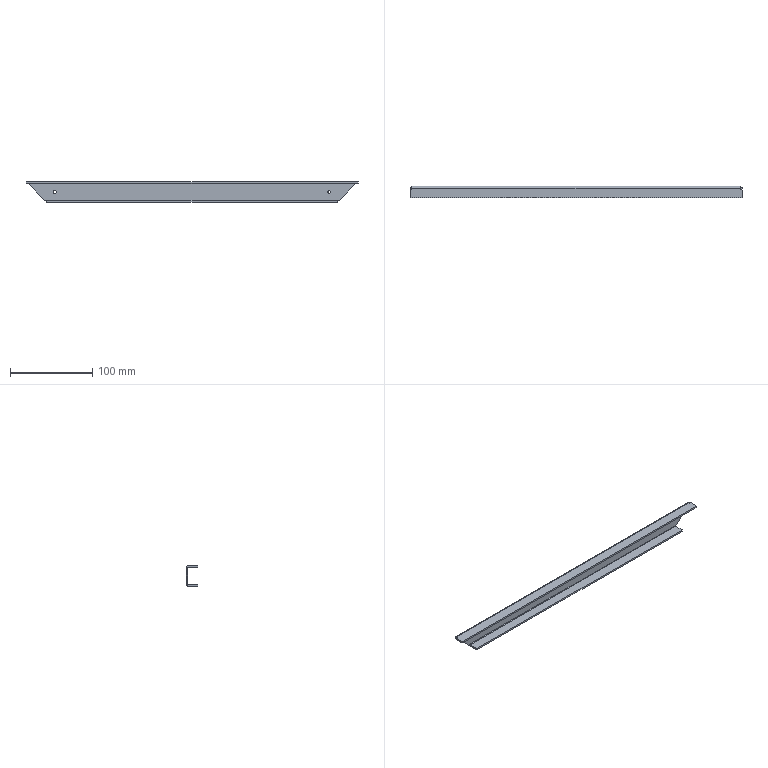Part | STEP file | Right Door Upper Clamp Rib Weldment | 1 solid | 33 faces | box 403 x 14 x 25 mm | volume 35999 mm3 | plane 25 | cylinder 8 | commonest cylinder face diameters 1 x2 3.2 x2 3.5 x2 5 x2
STEP:
#1=CARTESIAN_POINT('',(-215.258,8.055,-14.25));
#2=VERTEX_POINT('',#1);
#3=CARTESIAN_POINT('',(-215.258,8.055,-10.75));
#4=VERTEX_POINT('',#3);
#5=CARTESIAN_POINT('',(-215.258,8.055,-12.5));
#6=DIRECTION('',(0.,1.,0.));
#7=DIRECTION('',(0.,0.,1.));
#8=AXIS2_PLACEMENT_3D('',#5,#6,#7);
#9=CIRCLE('',#8,1.75);
#10=EDGE_CURVE('',#2,#4,#9,.T.);
#11=ORIENTED_EDGE('',*,*,#10,.F.);
#12=CARTESIAN_POINT('',(-215.258,10.055,-14.25));
#13=VERTEX_POINT('',#12);
#14=CARTESIAN_POINT('',(-215.258,0.05523,-14.25));
#15=DIRECTION('',(0.,1.,0.));
#16=VECTOR('',#15,1000.);
#17=LINE('',#14,#16);
#18=EDGE_CURVE('',#2,#13,#17,.T.);
#19=ORIENTED_EDGE('',*,*,#18,.T.);
#20=CARTESIAN_POINT('',(-215.258,10.055,-10.75));
#21=VERTEX_POINT('',#20);
#22=CARTESIAN_POINT('',(-215.258,10.055,-12.5));
#23=DIRECTION('',(0.,-1.,0.));
#24=DIRECTION('',(0.,0.,1.));
#25=AXIS2_PLACEMENT_3D('',#22,#23,#24);
#26=CIRCLE('',#25,1.75);
#27=EDGE_CURVE('',#21,#13,#26,.T.);
#28=ORIENTED_EDGE('',*,*,#27,.F.);
#29=CARTESIAN_POINT('',(-215.258,0.05523,-10.75));
#30=DIRECTION('',(0.,1.,0.));
#31=VECTOR('',#30,1000.);
#32=LINE('',#29,#31);
#33=EDGE_CURVE('',#4,#21,#32,.T.);
#34=ORIENTED_EDGE('',*,*,#33,.F.);
#35=EDGE_LOOP('',(#11,#19,#28,#34));
#36=FACE_OUTER_BOUND('',#35,.T.);
#37=CARTESIAN_POINT('',(-215.258,0.05523,-12.5));
#38=DIRECTION('',(0.,1.,0.));
#39=DIRECTION('',(0.,0.,1.));
#40=AXIS2_PLACEMENT_3D('',#37,#38,#39);
#41=CYLINDRICAL_SURFACE('',#40,1.75);
#42=ADVANCED_FACE('',(#36),#41,.F.);
#43=CARTESIAN_POINT('',(117.742,8.055,-14.1));
#44=VERTEX_POINT('',#43);
#45=CARTESIAN_POINT('',(117.742,8.055,-10.9));
#46=VERTEX_POINT('',#45);
#47=CARTESIAN_POINT('',(117.742,8.055,-12.5));
#48=DIRECTION('',(0.,1.,0.));
#49=DIRECTION('',(0.,0.,1.));
#50=AXIS2_PLACEMENT_3D('',#47,#48,#49);
#51=CIRCLE('',#50,1.6);
#52=EDGE_CURVE('',#44,#46,#51,.T.);
#53=ORIENTED_EDGE('',*,*,#52,.F.);
#54=CARTESIAN_POINT('',(117.742,10.055,-14.1));
#55=VERTEX_POINT('',#54);
#56=CARTESIAN_POINT('',(117.742,0.05523,-14.1));
#57=DIRECTION('',(0.,1.,0.));
#58=VECTOR('',#57,1000.);
#59=LINE('',#56,#58);
#60=EDGE_CURVE('',#44,#55,#59,.T.);
#61=ORIENTED_EDGE('',*,*,#60,.T.);
#62=CARTESIAN_POINT('',(117.742,10.055,-10.9));
#63=VERTEX_POINT('',#62);
#64=CARTESIAN_POINT('',(117.742,10.055,-12.5));
#65=DIRECTION('',(0.,-1.,0.));
#66=DIRECTION('',(0.,0.,1.));
#67=AXIS2_PLACEMENT_3D('',#64,#65,#66);
#68=CIRCLE('',#67,1.6);
#69=EDGE_CURVE('',#63,#55,#68,.T.);
#70=ORIENTED_EDGE('',*,*,#69,.F.);
#71=CARTESIAN_POINT('',(117.742,0.05523,-10.9));
#72=DIRECTION('',(0.,1.,0.));
#73=VECTOR('',#72,1000.);
#74=LINE('',#71,#73);
#75=EDGE_CURVE('',#46,#63,#74,.T.);
#76=ORIENTED_EDGE('',*,*,#75,.F.);
#77=EDGE_LOOP('',(#53,#61,#70,#76));
#78=FACE_OUTER_BOUND('',#77,.T.);
#79=CARTESIAN_POINT('',(117.742,0.05523,-12.5));
#80=DIRECTION('',(0.,1.,0.));
#81=DIRECTION('',(0.,0.,1.));
#82=AXIS2_PLACEMENT_3D('',#79,#80,#81);
#83=CYLINDRICAL_SURFACE('',#82,1.6);
#84=ADVANCED_FACE('',(#78),#83,.F.);
#85=ORIENTED_EDGE('',*,*,#27,.T.);
#86=CARTESIAN_POINT('',(-215.258,10.055,-12.5));
#87=DIRECTION('',(0.,-1.,0.));
#88=DIRECTION('',(0.,0.,1.));
#89=AXIS2_PLACEMENT_3D('',#86,#87,#88);
#90=CIRCLE('',#89,1.75);
#91=EDGE_CURVE('',#13,#21,#90,.T.);
#92=ORIENTED_EDGE('',*,*,#91,.T.);
#93=EDGE_LOOP('',(#85,#92));
#94=FACE_BOUND('',#93,.T.);
#95=ORIENTED_EDGE('',*,*,#69,.T.);
#96=CARTESIAN_POINT('',(117.742,10.055,-12.5));
#97=DIRECTION('',(0.,-1.,0.));
#98=DIRECTION('',(0.,0.,1.));
#99=AXIS2_PLACEMENT_3D('',#96,#97,#98);
#100=CIRCLE('',#99,1.6);
#101=EDGE_CURVE('',#55,#63,#100,.T.);
#102=ORIENTED_EDGE('',*,*,#101,.T.);
#103=EDGE_LOOP('',(#95,#102));
#104=FACE_BOUND('',#103,.T.);
#105=CARTESIAN_POINT('',(130.142,10.055,-22.5));
#106=VERTEX_POINT('',#105);
#107=CARTESIAN_POINT('',(127.642,10.055,-22.5));
#108=VERTEX_POINT('',#107);
#109=CARTESIAN_POINT('',(0.,10.055,-22.5));
#110=DIRECTION('',(-1.,0.,0.));
#111=VECTOR('',#110,1000.);
#112=LINE('',#109,#111);
#113=EDGE_CURVE('',#106,#108,#112,.T.);
#114=ORIENTED_EDGE('',*,*,#113,.T.);
#115=CARTESIAN_POINT('',(-225.158,10.055,-22.5));
#116=VERTEX_POINT('',#115);
#117=CARTESIAN_POINT('',(0.,10.055,-22.5));
#118=DIRECTION('',(-1.,0.,0.));
#119=VECTOR('',#118,1000.);
#120=LINE('',#117,#119);
#121=EDGE_CURVE('',#108,#116,#120,.T.);
#122=ORIENTED_EDGE('',*,*,#121,.T.);
#123=CARTESIAN_POINT('',(-227.654,10.055,-22.5));
#124=VERTEX_POINT('',#123);
#125=CARTESIAN_POINT('',(0.,10.055,-22.5));
#126=DIRECTION('',(-1.,0.,0.));
#127=VECTOR('',#126,1000.);
#128=LINE('',#125,#127);
#129=EDGE_CURVE('',#116,#124,#128,.T.);
#130=ORIENTED_EDGE('',*,*,#129,.T.);
#131=CARTESIAN_POINT('',(-227.654,10.055,-22.505));
#132=VERTEX_POINT('',#131);
#133=CARTESIAN_POINT('',(-227.654,10.055,-22.5));
#134=DIRECTION('',(0.,0.,-1.));
#135=VECTOR('',#134,1000.);
#136=LINE('',#133,#135);
#137=EDGE_CURVE('',#124,#132,#136,.T.);
#138=ORIENTED_EDGE('',*,*,#137,.T.);
#139=CARTESIAN_POINT('',(-247.658,10.055,-2.5));
#140=VERTEX_POINT('',#139);
#141=CARTESIAN_POINT('',(-227.654,10.055,-22.505));
#142=DIRECTION('',(-0.7071,0.,0.7071));
#143=VECTOR('',#142,1000.);
#144=LINE('',#141,#143);
#145=EDGE_CURVE('',#132,#140,#144,.T.);
#146=ORIENTED_EDGE('',*,*,#145,.T.);
#147=CARTESIAN_POINT('',(150.142,10.055,-2.5));
#148=VERTEX_POINT('',#147);
#149=CARTESIAN_POINT('',(0.,10.055,-2.5));
#150=DIRECTION('',(1.,0.,0.));
#151=VECTOR('',#150,1000.);
#152=LINE('',#149,#151);
#153=EDGE_CURVE('',#140,#148,#152,.T.);
#154=ORIENTED_EDGE('',*,*,#153,.T.);
#155=CARTESIAN_POINT('',(150.142,10.055,-2.5));
#156=DIRECTION('',(-0.7071,0.,-0.7071));
#157=VECTOR('',#156,1000.);
#158=LINE('',#155,#157);
#159=EDGE_CURVE('',#148,#106,#158,.T.);
#160=ORIENTED_EDGE('',*,*,#159,.T.);
#161=EDGE_LOOP('',(#114,#122,#130,#138,#146,#154,#160));
#162=FACE_OUTER_BOUND('',#161,.T.);
#163=CARTESIAN_POINT('',(0.,10.055,0.));
#164=DIRECTION('',(0.,1.,0.));
#165=DIRECTION('',(0.,0.,1.));
#166=AXIS2_PLACEMENT_3D('',#163,#164,#165);
#167=PLANE('',#166);
#168=ADVANCED_FACE('',(#94,#104,#162),#167,.T.);
#169=ORIENTED_EDGE('',*,*,#18,.F.);
#170=CARTESIAN_POINT('',(-215.258,8.055,-12.5));
#171=DIRECTION('',(0.,1.,0.));
#172=DIRECTION('',(0.,0.,1.));
#173=AXIS2_PLACEMENT_3D('',#170,#171,#172);
#174=CIRCLE('',#173,1.75);
#175=EDGE_CURVE('',#4,#2,#174,.T.);
#176=ORIENTED_EDGE('',*,*,#175,.F.);
#177=ORIENTED_EDGE('',*,*,#33,.T.);
#178=ORIENTED_EDGE('',*,*,#91,.F.);
#179=EDGE_LOOP('',(#169,#176,#177,#178));
#180=FACE_OUTER_BOUND('',#179,.T.);
#181=CARTESIAN_POINT('',(-215.258,0.05523,-12.5));
#182=DIRECTION('',(0.,1.,0.));
#183=DIRECTION('',(0.,0.,1.));
#184=AXIS2_PLACEMENT_3D('',#181,#182,#183);
#185=CYLINDRICAL_SURFACE('',#184,1.75);
#186=ADVANCED_FACE('',(#180),#185,.F.);
#187=ORIENTED_EDGE('',*,*,#60,.F.);
#188=CARTESIAN_POINT('',(117.742,8.055,-12.5));
#189=DIRECTION('',(0.,1.,0.));
#190=DIRECTION('',(0.,0.,1.));
#191=AXIS2_PLACEMENT_3D('',#188,#189,#190);
#192=CIRCLE('',#191,1.6);
#193=EDGE_CURVE('',#46,#44,#192,.T.);
#194=ORIENTED_EDGE('',*,*,#193,.F.);
#195=ORIENTED_EDGE('',*,*,#75,.T.);
#196=ORIENTED_EDGE('',*,*,#101,.F.);
#197=EDGE_LOOP('',(#187,#194,#195,#196));
#198=FACE_OUTER_BOUND('',#197,.T.);
#199=CARTESIAN_POINT('',(117.742,0.05523,-12.5));
#200=DIRECTION('',(0.,1.,0.));
#201=DIRECTION('',(0.,0.,1.));
#202=AXIS2_PLACEMENT_3D('',#199,#200,#201);
#203=CYLINDRICAL_SURFACE('',#202,1.6);
#204=ADVANCED_FACE('',(#198),#203,.F.);
#205=CARTESIAN_POINT('',(127.642,7.555,-25.));
#206=VERTEX_POINT('',#205);
#207=CARTESIAN_POINT('',(-225.158,7.555,-25.));
#208=VERTEX_POINT('',#207);
#209=CARTESIAN_POINT('',(127.642,7.555,-25.));
#210=DIRECTION('',(-1.,0.,0.));
#211=VECTOR('',#210,1000.);
#212=LINE('',#209,#211);
#213=EDGE_CURVE('',#206,#208,#212,.T.);
#214=ORIENTED_EDGE('',*,*,#213,.T.);
#215=CARTESIAN_POINT('',(-225.158,7.555,-22.5));
#216=DIRECTION('',(1.,0.,0.));
#217=DIRECTION('',(0.,0.,-1.));
#218=AXIS2_PLACEMENT_3D('',#215,#216,#217);
#219=CIRCLE('',#218,2.5);
#220=EDGE_CURVE('',#208,#116,#219,.T.);
#221=ORIENTED_EDGE('',*,*,#220,.T.);
#222=ORIENTED_EDGE('',*,*,#121,.F.);
#223=CARTESIAN_POINT('',(127.642,7.555,-22.5));
#224=DIRECTION('',(-1.,0.,0.));
#225=DIRECTION('',(0.,0.,-1.));
#226=AXIS2_PLACEMENT_3D('',#223,#224,#225);
#227=CIRCLE('',#226,2.5);
#228=EDGE_CURVE('',#108,#206,#227,.T.);
#229=ORIENTED_EDGE('',*,*,#228,.T.);
#230=EDGE_LOOP('',(#214,#221,#222,#229));
#231=FACE_OUTER_BOUND('',#230,.T.);
#232=CARTESIAN_POINT('',(127.642,7.555,-22.5));
#233=DIRECTION('',(1.,0.,0.));
#234=DIRECTION('',(0.,0.,-1.));
#235=AXIS2_PLACEMENT_3D('',#232,#233,#234);
#236=CYLINDRICAL_SURFACE('',#235,2.5);
#237=ADVANCED_FACE('',(#231),#236,.T.);
#238=ORIENTED_EDGE('',*,*,#113,.F.);
#239=CARTESIAN_POINT('',(130.142,8.055,-22.5));
#240=VERTEX_POINT('',#239);
#241=CARTESIAN_POINT('',(130.142,0.05523,-22.5));
#242=DIRECTION('',(0.,1.,0.));
#243=VECTOR('',#242,1000.);
#244=LINE('',#241,#243);
#245=EDGE_CURVE('',#240,#106,#244,.T.);
#246=ORIENTED_EDGE('',*,*,#245,.F.);
#247=CARTESIAN_POINT('',(127.642,8.055,-22.5));
#248=VERTEX_POINT('',#247);
#249=CARTESIAN_POINT('',(127.642,8.055,-22.5));
#250=DIRECTION('',(1.,0.,0.));
#251=VECTOR('',#250,1000.);
#252=LINE('',#249,#251);
#253=EDGE_CURVE('',#248,#240,#252,.T.);
#254=ORIENTED_EDGE('',*,*,#253,.F.);
#255=CARTESIAN_POINT('',(127.642,0.05523,-22.5));
#256=DIRECTION('',(0.,-1.,0.));
#257=VECTOR('',#256,1000.);
#258=LINE('',#255,#257);
#259=EDGE_CURVE('',#108,#248,#258,.T.);
#260=ORIENTED_EDGE('',*,*,#259,.F.);
#261=EDGE_LOOP('',(#238,#246,#254,#260));
#262=FACE_OUTER_BOUND('',#261,.T.);
#263=CARTESIAN_POINT('',(127.642,0.05523,-22.5));
#264=DIRECTION('',(0.,0.,1.));
#265=DIRECTION('',(0.,-1.,0.));
#266=AXIS2_PLACEMENT_3D('',#263,#264,#265);
#267=PLANE('',#266);
#268=ADVANCED_FACE('',(#262),#267,.F.);
#269=CARTESIAN_POINT('',(150.542,7.855,-2.1));
#270=VERTEX_POINT('',#269);
#271=CARTESIAN_POINT('',(150.142,8.055,-2.5));
#272=VERTEX_POINT('',#271);
#273=CARTESIAN_POINT('',(150.542,7.855,-2.1));
#274=CARTESIAN_POINT('',(150.445,7.984,-2.196));
#275=CARTESIAN_POINT('',(150.302,8.055,-2.34));
#276=CARTESIAN_POINT('',(150.142,8.055,-2.5));
#277=(BOUNDED_CURVE()B_SPLINE_CURVE(3,(#273,#274,#275,#276),.UNSPECIFIED.,.F.,.F.)B_SPLINE_CURVE_WITH_KNOTS((4,4),(0.6435,1.571),.UNSPECIFIED.)CURVE()GEOMETRIC_REPRESENTATION_ITEM()RATIONAL_B_SPLINE_CURVE((1.,0.9296,0.9296,1.))REPRESENTATION_ITEM(''));
#278=EDGE_CURVE('',#270,#272,#277,.T.);
#279=ORIENTED_EDGE('',*,*,#278,.T.);
#280=CARTESIAN_POINT('',(127.642,8.055,-25.));
#281=DIRECTION('',(-0.7071,0.,-0.7071));
#282=VECTOR('',#281,1000.);
#283=LINE('',#280,#282);
#284=EDGE_CURVE('',#272,#240,#283,.T.);
#285=ORIENTED_EDGE('',*,*,#284,.T.);
#286=ORIENTED_EDGE('',*,*,#245,.T.);
#287=ORIENTED_EDGE('',*,*,#159,.F.);
#288=CARTESIAN_POINT('',(150.542,10.023,-2.1));
#289=VERTEX_POINT('',#288);
#290=CARTESIAN_POINT('',(150.142,10.055,-2.5));
#291=CARTESIAN_POINT('',(150.276,10.055,-2.366));
#292=CARTESIAN_POINT('',(150.409,10.044,-2.232));
#293=CARTESIAN_POINT('',(150.542,10.023,-2.1));
#294=(BOUNDED_CURVE()B_SPLINE_CURVE(3,(#290,#291,#292,#293),.UNSPECIFIED.,.F.,.F.)B_SPLINE_CURVE_WITH_KNOTS((4,4),(4.712,4.873),.UNSPECIFIED.)CURVE()GEOMETRIC_REPRESENTATION_ITEM()RATIONAL_B_SPLINE_CURVE((1.,0.9978,0.9978,1.))REPRESENTATION_ITEM(''));
#295=EDGE_CURVE('',#148,#289,#294,.T.);
#296=ORIENTED_EDGE('',*,*,#295,.T.);
#297=CARTESIAN_POINT('',(150.542,10.055,-2.1));
#298=DIRECTION('',(0.,-1.,0.));
#299=VECTOR('',#298,1000.);
#300=LINE('',#297,#299);
#301=EDGE_CURVE('',#289,#270,#300,.T.);
#302=ORIENTED_EDGE('',*,*,#301,.T.);
#303=EDGE_LOOP('',(#279,#285,#286,#287,#296,#302));
#304=FACE_OUTER_BOUND('',#303,.T.);
#305=CARTESIAN_POINT('',(127.642,10.055,-25.));
#306=DIRECTION('',(0.7071,0.,-0.7071));
#307=DIRECTION('',(-0.7071,0.,-0.7071));
#308=AXIS2_PLACEMENT_3D('',#305,#306,#307);
#309=PLANE('',#308);
#310=ADVANCED_FACE('',(#304),#309,.T.);
#311=CARTESIAN_POINT('',(150.542,7.555,0.));
#312=VERTEX_POINT('',#311);
#313=CARTESIAN_POINT('',(150.542,7.555,-2.5));
#314=DIRECTION('',(-1.,0.,0.));
#315=DIRECTION('',(0.,0.,-1.));
#316=AXIS2_PLACEMENT_3D('',#313,#314,#315);
#317=CIRCLE('',#316,2.5);
#318=EDGE_CURVE('',#312,#289,#317,.T.);
#319=ORIENTED_EDGE('',*,*,#318,.T.);
#320=ORIENTED_EDGE('',*,*,#295,.F.);
#321=ORIENTED_EDGE('',*,*,#153,.F.);
#322=CARTESIAN_POINT('',(-248.058,10.023,-2.1));
#323=VERTEX_POINT('',#322);
#324=CARTESIAN_POINT('',(-247.658,10.055,-2.5));
#325=CARTESIAN_POINT('',(-247.792,10.055,-2.366));
#326=CARTESIAN_POINT('',(-247.926,10.044,-2.232));
#327=CARTESIAN_POINT('',(-248.058,10.023,-2.1));
#328=(BOUNDED_CURVE()B_SPLINE_CURVE(3,(#324,#325,#326,#327),.UNSPECIFIED.,.F.,.F.)B_SPLINE_CURVE_WITH_KNOTS((4,4),(1.571,1.731),.UNSPECIFIED.)CURVE()GEOMETRIC_REPRESENTATION_ITEM()RATIONAL_B_SPLINE_CURVE((1.,0.9978,0.9978,1.))REPRESENTATION_ITEM(''));
#329=EDGE_CURVE('',#140,#323,#328,.T.);
#330=ORIENTED_EDGE('',*,*,#329,.T.);
#331=CARTESIAN_POINT('',(-248.058,7.555,0.));
#332=VERTEX_POINT('',#331);
#333=CARTESIAN_POINT('',(-248.058,7.555,-2.5));
#334=DIRECTION('',(1.,0.,0.));
#335=DIRECTION('',(0.,0.,-1.));
#336=AXIS2_PLACEMENT_3D('',#333,#334,#335);
#337=CIRCLE('',#336,2.5);
#338=EDGE_CURVE('',#323,#332,#337,.T.);
#339=ORIENTED_EDGE('',*,*,#338,.T.);
#340=CARTESIAN_POINT('',(150.542,7.555,0.));
#341=DIRECTION('',(1.,0.,0.));
#342=VECTOR('',#341,1000.);
#343=LINE('',#340,#342);
#344=EDGE_CURVE('',#332,#312,#343,.T.);
#345=ORIENTED_EDGE('',*,*,#344,.T.);
#346=EDGE_LOOP('',(#319,#320,#321,#330,#339,#345));
#347=FACE_OUTER_BOUND('',#346,.T.);
#348=CARTESIAN_POINT('',(150.542,7.555,-2.5));
#349=DIRECTION('',(1.,0.,0.));
#350=DIRECTION('',(0.,0.,-1.));
#351=AXIS2_PLACEMENT_3D('',#348,#349,#350);
#352=CYLINDRICAL_SURFACE('',#351,2.5);
#353=ADVANCED_FACE('',(#347),#352,.T.);
#354=CARTESIAN_POINT('',(-247.658,8.055,-2.5));
#355=VERTEX_POINT('',#354);
#356=CARTESIAN_POINT('',(-227.654,8.055,-22.505));
#357=VERTEX_POINT('',#356);
#358=CARTESIAN_POINT('',(-248.058,8.055,-2.1));
#359=DIRECTION('',(0.7071,0.,-0.7071));
#360=VECTOR('',#359,1000.);
#361=LINE('',#358,#360);
#362=EDGE_CURVE('',#355,#357,#361,.T.);
#363=ORIENTED_EDGE('',*,*,#362,.F.);
#364=CARTESIAN_POINT('',(-248.058,7.855,-2.1));
#365=VERTEX_POINT('',#364);
#366=CARTESIAN_POINT('',(-247.658,8.055,-2.5));
#367=CARTESIAN_POINT('',(-247.819,8.055,-2.34));
#368=CARTESIAN_POINT('',(-247.962,7.984,-2.196));
#369=CARTESIAN_POINT('',(-248.058,7.855,-2.1));
#370=(BOUNDED_CURVE()B_SPLINE_CURVE(3,(#366,#367,#368,#369),.UNSPECIFIED.,.F.,.F.)B_SPLINE_CURVE_WITH_KNOTS((4,4),(1.571,2.498),.UNSPECIFIED.)CURVE()GEOMETRIC_REPRESENTATION_ITEM()RATIONAL_B_SPLINE_CURVE((1.,0.9296,0.9296,1.))REPRESENTATION_ITEM(''));
#371=EDGE_CURVE('',#355,#365,#370,.T.);
#372=ORIENTED_EDGE('',*,*,#371,.T.);
#373=CARTESIAN_POINT('',(-248.058,7.555,-2.1));
#374=DIRECTION('',(0.,-1.,0.));
#375=VECTOR('',#374,1000.);
#376=LINE('',#373,#375);
#377=EDGE_CURVE('',#323,#365,#376,.T.);
#378=ORIENTED_EDGE('',*,*,#377,.F.);
#379=ORIENTED_EDGE('',*,*,#329,.F.);
#380=ORIENTED_EDGE('',*,*,#145,.F.);
#381=CARTESIAN_POINT('',(-227.654,7.555,-22.505));
#382=DIRECTION('',(0.,1.,0.));
#383=VECTOR('',#382,1000.);
#384=LINE('',#381,#383);
#385=EDGE_CURVE('',#357,#132,#384,.T.);
#386=ORIENTED_EDGE('',*,*,#385,.F.);
#387=EDGE_LOOP('',(#363,#372,#378,#379,#380,#386));
#388=FACE_OUTER_BOUND('',#387,.T.);
#389=CARTESIAN_POINT('',(-248.058,7.555,-2.1));
#390=DIRECTION('',(0.7071,0.,0.7071));
#391=DIRECTION('',(0.7071,0.,-0.7071));
#392=AXIS2_PLACEMENT_3D('',#389,#390,#391);
#393=PLANE('',#392);
#394=ADVANCED_FACE('',(#388),#393,.F.);
#395=ORIENTED_EDGE('',*,*,#129,.F.);
#396=CARTESIAN_POINT('',(-225.158,8.055,-22.5));
#397=VERTEX_POINT('',#396);
#398=CARTESIAN_POINT('',(-225.158,0.05523,-22.5));
#399=DIRECTION('',(0.,1.,0.));
#400=VECTOR('',#399,1000.);
#401=LINE('',#398,#400);
#402=EDGE_CURVE('',#397,#116,#401,.T.);
#403=ORIENTED_EDGE('',*,*,#402,.F.);
#404=CARTESIAN_POINT('',(-227.654,8.055,-22.5));
#405=VERTEX_POINT('',#404);
#406=CARTESIAN_POINT('',(-225.158,8.055,-22.5));
#407=DIRECTION('',(1.,0.,0.));
#408=VECTOR('',#407,1000.);
#409=LINE('',#406,#408);
#410=EDGE_CURVE('',#405,#397,#409,.T.);
#411=ORIENTED_EDGE('',*,*,#410,.F.);
#412=CARTESIAN_POINT('',(-227.654,0.05523,-22.5));
#413=DIRECTION('',(0.,-1.,0.));
#414=VECTOR('',#413,1000.);
#415=LINE('',#412,#414);
#416=EDGE_CURVE('',#124,#405,#415,.T.);
#417=ORIENTED_EDGE('',*,*,#416,.F.);
#418=EDGE_LOOP('',(#395,#403,#411,#417));
#419=FACE_OUTER_BOUND('',#418,.T.);
#420=CARTESIAN_POINT('',(-225.158,0.05523,-22.5));
#421=DIRECTION('',(0.,0.,1.));
#422=DIRECTION('',(0.,-1.,0.));
#423=AXIS2_PLACEMENT_3D('',#420,#421,#422);
#424=PLANE('',#423);
#425=ADVANCED_FACE('',(#419),#424,.F.);
#426=ORIENTED_EDGE('',*,*,#410,.T.);
#427=CARTESIAN_POINT('',(0.,8.055,-22.5));
#428=DIRECTION('',(-1.,0.,0.));
#429=VECTOR('',#428,1000.);
#430=LINE('',#427,#429);
#431=EDGE_CURVE('',#248,#397,#430,.T.);
#432=ORIENTED_EDGE('',*,*,#431,.F.);
#433=ORIENTED_EDGE('',*,*,#253,.T.);
#434=ORIENTED_EDGE('',*,*,#284,.F.);
#435=CARTESIAN_POINT('',(0.,8.055,-2.5));
#436=DIRECTION('',(1.,0.,0.));
#437=VECTOR('',#436,1000.);
#438=LINE('',#435,#437);
#439=EDGE_CURVE('',#355,#272,#438,.T.);
#440=ORIENTED_EDGE('',*,*,#439,.F.);
#441=ORIENTED_EDGE('',*,*,#362,.T.);
#442=CARTESIAN_POINT('',(-227.654,8.055,0.));
#443=DIRECTION('',(0.,0.,-1.));
#444=VECTOR('',#443,1000.);
#445=LINE('',#442,#444);
#446=EDGE_CURVE('',#405,#357,#445,.T.);
#447=ORIENTED_EDGE('',*,*,#446,.F.);
#448=EDGE_LOOP('',(#426,#432,#433,#434,#440,#441,#447));
#449=FACE_OUTER_BOUND('',#448,.T.);
#450=ORIENTED_EDGE('',*,*,#175,.T.);
#451=ORIENTED_EDGE('',*,*,#10,.T.);
#452=EDGE_LOOP('',(#450,#451));
#453=FACE_BOUND('',#452,.T.);
#454=ORIENTED_EDGE('',*,*,#193,.T.);
#455=ORIENTED_EDGE('',*,*,#52,.T.);
#456=EDGE_LOOP('',(#454,#455));
#457=FACE_BOUND('',#456,.T.);
#458=CARTESIAN_POINT('',(0.,8.055,0.));
#459=DIRECTION('',(0.,1.,0.));
#460=DIRECTION('',(0.,0.,1.));
#461=AXIS2_PLACEMENT_3D('',#458,#459,#460);
#462=PLANE('',#461);
#463=ADVANCED_FACE('',(#449,#453,#457),#462,.F.);
#464=CARTESIAN_POINT('',(-225.158,-3.945,-25.));
#465=VERTEX_POINT('',#464);
#466=CARTESIAN_POINT('',(-225.158,-3.945,-23.));
#467=VERTEX_POINT('',#466);
#468=CARTESIAN_POINT('',(-225.158,-3.945,-22.5));
#469=DIRECTION('',(0.,0.,1.));
#470=VECTOR('',#469,1000.);
#471=LINE('',#468,#470);
#472=EDGE_CURVE('',#465,#467,#471,.T.);
#473=ORIENTED_EDGE('',*,*,#472,.T.);
#474=CARTESIAN_POINT('',(-225.158,7.555,-23.));
#475=VERTEX_POINT('',#474);
#476=CARTESIAN_POINT('',(-225.158,7.555,-23.));
#477=DIRECTION('',(0.,1.,0.));
#478=VECTOR('',#477,1000.);
#479=LINE('',#476,#478);
#480=EDGE_CURVE('',#467,#475,#479,.T.);
#481=ORIENTED_EDGE('',*,*,#480,.T.);
#482=CARTESIAN_POINT('',(-225.158,7.555,-22.5));
#483=DIRECTION('',(1.,0.,0.));
#484=DIRECTION('',(0.,0.,-1.));
#485=AXIS2_PLACEMENT_3D('',#482,#483,#484);
#486=CIRCLE('',#485,0.5);
#487=EDGE_CURVE('',#475,#397,#486,.T.);
#488=ORIENTED_EDGE('',*,*,#487,.T.);
#489=ORIENTED_EDGE('',*,*,#402,.T.);
#490=ORIENTED_EDGE('',*,*,#220,.F.);
#491=CARTESIAN_POINT('',(-225.158,7.555,-25.));
#492=DIRECTION('',(0.,-1.,0.));
#493=VECTOR('',#492,1000.);
#494=LINE('',#491,#493);
#495=EDGE_CURVE('',#208,#465,#494,.T.);
#496=ORIENTED_EDGE('',*,*,#495,.T.);
#497=EDGE_LOOP('',(#473,#481,#488,#489,#490,#496));
#498=FACE_OUTER_BOUND('',#497,.T.);
#499=CARTESIAN_POINT('',(-225.158,7.555,-22.5));
#500=DIRECTION('',(-1.,0.,0.));
#501=DIRECTION('',(0.,0.,1.));
#502=AXIS2_PLACEMENT_3D('',#499,#500,#501);
#503=PLANE('',#502);
#504=ADVANCED_FACE('',(#498),#503,.T.);
#505=CARTESIAN_POINT('',(127.642,-3.945,-25.));
#506=VERTEX_POINT('',#505);
#507=CARTESIAN_POINT('',(127.642,0.,-25.));
#508=DIRECTION('',(0.,-1.,0.));
#509=VECTOR('',#508,1000.);
#510=LINE('',#507,#509);
#511=EDGE_CURVE('',#206,#506,#510,.T.);
#512=ORIENTED_EDGE('',*,*,#511,.T.);
#513=CARTESIAN_POINT('',(0.,-3.945,-25.));
#514=DIRECTION('',(-1.,0.,0.));
#515=VECTOR('',#514,1000.);
#516=LINE('',#513,#515);
#517=EDGE_CURVE('',#506,#465,#516,.T.);
#518=ORIENTED_EDGE('',*,*,#517,.T.);
#519=ORIENTED_EDGE('',*,*,#495,.F.);
#520=ORIENTED_EDGE('',*,*,#213,.F.);
#521=EDGE_LOOP('',(#512,#518,#519,#520));
#522=FACE_OUTER_BOUND('',#521,.T.);
#523=CARTESIAN_POINT('',(0.,0.,-25.));
#524=DIRECTION('',(0.,0.,-1.));
#525=DIRECTION('',(0.,1.,0.));
#526=AXIS2_PLACEMENT_3D('',#523,#524,#525);
#527=PLANE('',#526);
#528=ADVANCED_FACE('',(#522),#527,.T.);
#529=ORIENTED_EDGE('',*,*,#228,.F.);
#530=ORIENTED_EDGE('',*,*,#259,.T.);
#531=CARTESIAN_POINT('',(127.642,7.555,-23.));
#532=VERTEX_POINT('',#531);
#533=CARTESIAN_POINT('',(127.642,7.555,-22.5));
#534=DIRECTION('',(1.,0.,0.));
#535=DIRECTION('',(0.,0.,-1.));
#536=AXIS2_PLACEMENT_3D('',#533,#534,#535);
#537=CIRCLE('',#536,0.5);
#538=EDGE_CURVE('',#532,#248,#537,.T.);
#539=ORIENTED_EDGE('',*,*,#538,.F.);
#540=CARTESIAN_POINT('',(127.642,-3.945,-23.));
#541=VERTEX_POINT('',#540);
#542=CARTESIAN_POINT('',(127.642,7.555,-23.));
#543=DIRECTION('',(0.,1.,0.));
#544=VECTOR('',#543,1000.);
#545=LINE('',#542,#544);
#546=EDGE_CURVE('',#541,#532,#545,.T.);
#547=ORIENTED_EDGE('',*,*,#546,.F.);
#548=CARTESIAN_POINT('',(127.642,-3.945,-22.5));
#549=DIRECTION('',(0.,0.,1.));
#550=VECTOR('',#549,1000.);
#551=LINE('',#548,#550);
#552=EDGE_CURVE('',#506,#541,#551,.T.);
#553=ORIENTED_EDGE('',*,*,#552,.F.);
#554=ORIENTED_EDGE('',*,*,#511,.F.);
#555=EDGE_LOOP('',(#529,#530,#539,#547,#553,#554));
#556=FACE_OUTER_BOUND('',#555,.T.);
#557=CARTESIAN_POINT('',(127.642,7.555,-22.5));
#558=DIRECTION('',(-1.,0.,0.));
#559=DIRECTION('',(0.,0.,1.));
#560=AXIS2_PLACEMENT_3D('',#557,#558,#559);
#561=PLANE('',#560);
#562=ADVANCED_FACE('',(#556),#561,.F.);
#563=ORIENTED_EDGE('',*,*,#301,.F.);
#564=ORIENTED_EDGE('',*,*,#318,.F.);
#565=CARTESIAN_POINT('',(150.542,6.555,0.));
#566=VERTEX_POINT('',#565);
#567=CARTESIAN_POINT('',(150.542,0.,0.));
#568=DIRECTION('',(0.,1.,0.));
#569=VECTOR('',#568,1000.);
#570=LINE('',#567,#569);
#571=EDGE_CURVE('',#566,#312,#570,.T.);
#572=ORIENTED_EDGE('',*,*,#571,.F.);
#573=CARTESIAN_POINT('',(150.542,6.555,-2.));
#574=VERTEX_POINT('',#573);
#575=CARTESIAN_POINT('',(150.542,6.555,-2.));
#576=DIRECTION('',(0.,0.,-1.));
#577=VECTOR('',#576,1000.);
#578=LINE('',#575,#577);
#579=EDGE_CURVE('',#566,#574,#578,.T.);
#580=ORIENTED_EDGE('',*,*,#579,.T.);
#581=CARTESIAN_POINT('',(150.542,7.555,-2.));
#582=VERTEX_POINT('',#581);
#583=CARTESIAN_POINT('',(150.542,6.555,-2.));
#584=DIRECTION('',(0.,1.,0.));
#585=VECTOR('',#584,1000.);
#586=LINE('',#583,#585);
#587=EDGE_CURVE('',#574,#582,#586,.T.);
#588=ORIENTED_EDGE('',*,*,#587,.T.);
#589=CARTESIAN_POINT('',(150.542,7.555,-2.5));
#590=DIRECTION('',(1.,0.,0.));
#591=DIRECTION('',(0.,0.,-1.));
#592=AXIS2_PLACEMENT_3D('',#589,#590,#591);
#593=CIRCLE('',#592,0.5);
#594=EDGE_CURVE('',#270,#582,#593,.T.);
#595=ORIENTED_EDGE('',*,*,#594,.F.);
#596=EDGE_LOOP('',(#563,#564,#572,#580,#588,#595));
#597=FACE_OUTER_BOUND('',#596,.T.);
#598=CARTESIAN_POINT('',(150.542,7.555,-2.5));
#599=DIRECTION('',(-1.,0.,0.));
#600=DIRECTION('',(0.,0.,1.));
#601=AXIS2_PLACEMENT_3D('',#598,#599,#600);
#602=PLANE('',#601);
#603=ADVANCED_FACE('',(#597),#602,.F.);
#604=CARTESIAN_POINT('',(-250.258,-3.945,0.));
#605=VERTEX_POINT('',#604);
#606=CARTESIAN_POINT('',(152.742,-3.945,0.));
#607=VERTEX_POINT('',#606);
#608=CARTESIAN_POINT('',(0.,-3.945,0.));
#609=DIRECTION('',(1.,0.,0.));
#610=VECTOR('',#609,1000.);
#611=LINE('',#608,#610);
#612=EDGE_CURVE('',#605,#607,#611,.T.);
#613=ORIENTED_EDGE('',*,*,#612,.T.);
#614=CARTESIAN_POINT('',(152.742,8.055,0.));
#615=VERTEX_POINT('',#614);
#616=CARTESIAN_POINT('',(152.742,0.,0.));
#617=DIRECTION('',(0.,1.,0.));
#618=VECTOR('',#617,1000.);
#619=LINE('',#616,#618);
#620=EDGE_CURVE('',#607,#615,#619,.T.);
#621=ORIENTED_EDGE('',*,*,#620,.T.);
#622=CARTESIAN_POINT('',(151.542,8.055,0.));
#623=VERTEX_POINT('',#622);
#624=CARTESIAN_POINT('',(152.742,8.055,0.));
#625=DIRECTION('',(-1.,0.,0.));
#626=VECTOR('',#625,1000.);
#627=LINE('',#624,#626);
#628=EDGE_CURVE('',#615,#623,#627,.T.);
#629=ORIENTED_EDGE('',*,*,#628,.T.);
#630=CARTESIAN_POINT('',(151.542,6.555,0.));
#631=VERTEX_POINT('',#630);
#632=CARTESIAN_POINT('',(151.542,10.055,0.));
#633=DIRECTION('',(0.,1.,0.));
#634=VECTOR('',#633,1000.);
#635=LINE('',#632,#634);
#636=EDGE_CURVE('',#631,#623,#635,.T.);
#637=ORIENTED_EDGE('',*,*,#636,.F.);
#638=CARTESIAN_POINT('',(151.542,6.555,0.));
#639=DIRECTION('',(1.,0.,0.));
#640=VECTOR('',#639,1000.);
#641=LINE('',#638,#640);
#642=EDGE_CURVE('',#566,#631,#641,.T.);
#643=ORIENTED_EDGE('',*,*,#642,.F.);
#644=ORIENTED_EDGE('',*,*,#571,.T.);
#645=ORIENTED_EDGE('',*,*,#344,.F.);
#646=CARTESIAN_POINT('',(-248.058,6.555,0.));
#647=VERTEX_POINT('',#646);
#648=CARTESIAN_POINT('',(-248.058,7.555,0.));
#649=DIRECTION('',(0.,1.,0.));
#650=VECTOR('',#649,1000.);
#651=LINE('',#648,#650);
#652=EDGE_CURVE('',#647,#332,#651,.T.);
#653=ORIENTED_EDGE('',*,*,#652,.F.);
#654=CARTESIAN_POINT('',(-249.058,6.555,0.));
#655=VERTEX_POINT('',#654);
#656=CARTESIAN_POINT('',(-248.058,6.555,0.));
#657=DIRECTION('',(1.,0.,0.));
#658=VECTOR('',#657,1000.);
#659=LINE('',#656,#658);
#660=EDGE_CURVE('',#655,#647,#659,.T.);
#661=ORIENTED_EDGE('',*,*,#660,.F.);
#662=CARTESIAN_POINT('',(-249.058,8.055,0.));
#663=VERTEX_POINT('',#662);
#664=CARTESIAN_POINT('',(-249.058,6.555,0.));
#665=DIRECTION('',(0.,-1.,0.));
#666=VECTOR('',#665,1000.);
#667=LINE('',#664,#666);
#668=EDGE_CURVE('',#663,#655,#667,.T.);
#669=ORIENTED_EDGE('',*,*,#668,.F.);
#670=CARTESIAN_POINT('',(-250.258,8.055,0.));
#671=VERTEX_POINT('',#670);
#672=CARTESIAN_POINT('',(-250.258,8.055,0.));
#673=DIRECTION('',(-1.,0.,0.));
#674=VECTOR('',#673,1000.);
#675=LINE('',#672,#674);
#676=EDGE_CURVE('',#663,#671,#675,.T.);
#677=ORIENTED_EDGE('',*,*,#676,.T.);
#678=CARTESIAN_POINT('',(-250.258,0.,0.));
#679=DIRECTION('',(0.,-1.,0.));
#680=VECTOR('',#679,1000.);
#681=LINE('',#678,#680);
#682=EDGE_CURVE('',#671,#605,#681,.T.);
#683=ORIENTED_EDGE('',*,*,#682,.T.);
#684=EDGE_LOOP('',(#613,#621,#629,#637,#643,#644,#645,#653,#661,#669,#677,#683));
#685=FACE_OUTER_BOUND('',#684,.T.);
#686=CARTESIAN_POINT('',(0.,0.,0.));
#687=DIRECTION('',(0.,0.,1.));
#688=DIRECTION('',(1.,0.,0.));
#689=AXIS2_PLACEMENT_3D('',#686,#687,#688);
#690=PLANE('',#689);
#691=ADVANCED_FACE('',(#685),#690,.T.);
#692=CARTESIAN_POINT('',(-248.058,7.555,-2.));
#693=VERTEX_POINT('',#692);
#694=CARTESIAN_POINT('',(-248.058,7.555,-2.5));
#695=DIRECTION('',(1.,0.,0.));
#696=DIRECTION('',(0.,0.,-1.));
#697=AXIS2_PLACEMENT_3D('',#694,#695,#696);
#698=CIRCLE('',#697,0.5);
#699=EDGE_CURVE('',#365,#693,#698,.T.);
#700=ORIENTED_EDGE('',*,*,#699,.T.);
#701=CARTESIAN_POINT('',(-248.058,6.555,-2.));
#702=VERTEX_POINT('',#701);
#703=CARTESIAN_POINT('',(-248.058,7.555,-2.));
#704=DIRECTION('',(0.,-1.,0.));
#705=VECTOR('',#704,1000.);
#706=LINE('',#703,#705);
#707=EDGE_CURVE('',#693,#702,#706,.T.);
#708=ORIENTED_EDGE('',*,*,#707,.T.);
#709=CARTESIAN_POINT('',(-248.058,6.555,-2.));
#710=DIRECTION('',(0.,0.,1.));
#711=VECTOR('',#710,1000.);
#712=LINE('',#709,#711);
#713=EDGE_CURVE('',#702,#647,#712,.T.);
#714=ORIENTED_EDGE('',*,*,#713,.T.);
#715=ORIENTED_EDGE('',*,*,#652,.T.);
#716=ORIENTED_EDGE('',*,*,#338,.F.);
#717=ORIENTED_EDGE('',*,*,#377,.T.);
#718=EDGE_LOOP('',(#700,#708,#714,#715,#716,#717));
#719=FACE_OUTER_BOUND('',#718,.T.);
#720=CARTESIAN_POINT('',(-248.058,7.555,-2.5));
#721=DIRECTION('',(-1.,0.,0.));
#722=DIRECTION('',(0.,0.,1.));
#723=AXIS2_PLACEMENT_3D('',#720,#721,#722);
#724=PLANE('',#723);
#725=ADVANCED_FACE('',(#719),#724,.T.);
#726=ORIENTED_EDGE('',*,*,#137,.F.);
#727=ORIENTED_EDGE('',*,*,#416,.T.);
#728=ORIENTED_EDGE('',*,*,#446,.T.);
#729=ORIENTED_EDGE('',*,*,#385,.T.);
#730=EDGE_LOOP('',(#726,#727,#728,#729));
#731=FACE_OUTER_BOUND('',#730,.T.);
#732=CARTESIAN_POINT('',(-227.654,0.05523,-22.5));
#733=DIRECTION('',(-1.,0.,0.));
#734=DIRECTION('',(0.,-1.,0.));
#735=AXIS2_PLACEMENT_3D('',#732,#733,#734);
#736=PLANE('',#735);
#737=ADVANCED_FACE('',(#731),#736,.F.);
#738=ORIENTED_EDGE('',*,*,#487,.F.);
#739=CARTESIAN_POINT('',(127.642,7.555,-23.));
#740=DIRECTION('',(-1.,0.,0.));
#741=VECTOR('',#740,1000.);
#742=LINE('',#739,#741);
#743=EDGE_CURVE('',#532,#475,#742,.T.);
#744=ORIENTED_EDGE('',*,*,#743,.F.);
#745=ORIENTED_EDGE('',*,*,#538,.T.);
#746=ORIENTED_EDGE('',*,*,#431,.T.);
#747=EDGE_LOOP('',(#738,#744,#745,#746));
#748=FACE_OUTER_BOUND('',#747,.T.);
#749=CARTESIAN_POINT('',(127.642,7.555,-22.5));
#750=DIRECTION('',(1.,0.,0.));
#751=DIRECTION('',(0.,0.,-1.));
#752=AXIS2_PLACEMENT_3D('',#749,#750,#751);
#753=CYLINDRICAL_SURFACE('',#752,0.5);
#754=ADVANCED_FACE('',(#748),#753,.F.);
#755=ORIENTED_EDGE('',*,*,#371,.F.);
#756=ORIENTED_EDGE('',*,*,#439,.T.);
#757=ORIENTED_EDGE('',*,*,#278,.F.);
#758=ORIENTED_EDGE('',*,*,#594,.T.);
#759=CARTESIAN_POINT('',(150.542,7.555,-2.));
#760=DIRECTION('',(1.,0.,0.));
#761=VECTOR('',#760,1000.);
#762=LINE('',#759,#761);
#763=EDGE_CURVE('',#693,#582,#762,.T.);
#764=ORIENTED_EDGE('',*,*,#763,.F.);
#765=ORIENTED_EDGE('',*,*,#699,.F.);
#766=EDGE_LOOP('',(#755,#756,#757,#758,#764,#765));
#767=FACE_OUTER_BOUND('',#766,.T.);
#768=CARTESIAN_POINT('',(150.542,7.555,-2.5));
#769=DIRECTION('',(1.,0.,0.));
#770=DIRECTION('',(0.,0.,-1.));
#771=AXIS2_PLACEMENT_3D('',#768,#769,#770);
#772=CYLINDRICAL_SURFACE('',#771,0.5);
#773=ADVANCED_FACE('',(#767),#772,.F.);
#774=ORIENTED_EDGE('',*,*,#480,.F.);
#775=CARTESIAN_POINT('',(0.,-3.945,-23.));
#776=DIRECTION('',(-1.,0.,0.));
#777=VECTOR('',#776,1000.);
#778=LINE('',#775,#777);
#779=EDGE_CURVE('',#541,#467,#778,.T.);
#780=ORIENTED_EDGE('',*,*,#779,.F.);
#781=ORIENTED_EDGE('',*,*,#546,.T.);
#782=ORIENTED_EDGE('',*,*,#743,.T.);
#783=EDGE_LOOP('',(#774,#780,#781,#782));
#784=FACE_OUTER_BOUND('',#783,.T.);
#785=CARTESIAN_POINT('',(0.,0.,-23.));
#786=DIRECTION('',(0.,0.,-1.));
#787=DIRECTION('',(0.,1.,0.));
#788=AXIS2_PLACEMENT_3D('',#785,#786,#787);
#789=PLANE('',#788);
#790=ADVANCED_FACE('',(#784),#789,.F.);
#791=ORIENTED_EDGE('',*,*,#517,.F.);
#792=ORIENTED_EDGE('',*,*,#552,.T.);
#793=ORIENTED_EDGE('',*,*,#779,.T.);
#794=ORIENTED_EDGE('',*,*,#472,.F.);
#795=EDGE_LOOP('',(#791,#792,#793,#794));
#796=FACE_OUTER_BOUND('',#795,.T.);
#797=CARTESIAN_POINT('',(127.642,-3.945,-25.));
#798=DIRECTION('',(0.,-1.,0.));
#799=DIRECTION('',(0.,0.,-1.));
#800=AXIS2_PLACEMENT_3D('',#797,#798,#799);
#801=PLANE('',#800);
#802=ADVANCED_FACE('',(#796),#801,.T.);
#803=CARTESIAN_POINT('',(152.742,-3.945,-2.));
#804=VERTEX_POINT('',#803);
#805=CARTESIAN_POINT('',(152.742,-3.945,-2.));
#806=DIRECTION('',(0.,0.,-1.));
#807=VECTOR('',#806,1000.);
#808=LINE('',#805,#807);
#809=EDGE_CURVE('',#607,#804,#808,.T.);
#810=ORIENTED_EDGE('',*,*,#809,.T.);
#811=CARTESIAN_POINT('',(152.742,8.055,-2.));
#812=VERTEX_POINT('',#811);
#813=CARTESIAN_POINT('',(152.742,10.055,-2.));
#814=DIRECTION('',(0.,1.,0.));
#815=VECTOR('',#814,1000.);
#816=LINE('',#813,#815);
#817=EDGE_CURVE('',#804,#812,#816,.T.);
#818=ORIENTED_EDGE('',*,*,#817,.T.);
#819=CARTESIAN_POINT('',(152.742,8.055,-2.));
#820=DIRECTION('',(0.,0.,1.));
#821=VECTOR('',#820,1000.);
#822=LINE('',#819,#821);
#823=EDGE_CURVE('',#812,#615,#822,.T.);
#824=ORIENTED_EDGE('',*,*,#823,.T.);
#825=ORIENTED_EDGE('',*,*,#620,.F.);
#826=EDGE_LOOP('',(#810,#818,#824,#825));
#827=FACE_OUTER_BOUND('',#826,.T.);
#828=CARTESIAN_POINT('',(152.742,10.055,-2.));
#829=DIRECTION('',(1.,0.,0.));
#830=DIRECTION('',(0.,0.,-1.));
#831=AXIS2_PLACEMENT_3D('',#828,#829,#830);
#832=PLANE('',#831);
#833=ADVANCED_FACE('',(#827),#832,.T.);
#834=CARTESIAN_POINT('',(-250.258,-3.945,-2.));
#835=VERTEX_POINT('',#834);
#836=CARTESIAN_POINT('',(-250.258,-3.945,-2.));
#837=DIRECTION('',(1.,0.,0.));
#838=VECTOR('',#837,1000.);
#839=LINE('',#836,#838);
#840=EDGE_CURVE('',#835,#804,#839,.T.);
#841=ORIENTED_EDGE('',*,*,#840,.T.);
#842=ORIENTED_EDGE('',*,*,#809,.F.);
#843=ORIENTED_EDGE('',*,*,#612,.F.);
#844=CARTESIAN_POINT('',(-250.258,-3.945,-2.));
#845=DIRECTION('',(0.,0.,-1.));
#846=VECTOR('',#845,1000.);
#847=LINE('',#844,#846);
#848=EDGE_CURVE('',#605,#835,#847,.T.);
#849=ORIENTED_EDGE('',*,*,#848,.T.);
#850=EDGE_LOOP('',(#841,#842,#843,#849));
#851=FACE_OUTER_BOUND('',#850,.T.);
#852=CARTESIAN_POINT('',(-250.258,-3.945,-2.));
#853=DIRECTION('',(0.,-1.,0.));
#854=DIRECTION('',(1.,0.,0.));
#855=AXIS2_PLACEMENT_3D('',#852,#853,#854);
#856=PLANE('',#855);
#857=ADVANCED_FACE('',(#851),#856,.T.);
#858=ORIENTED_EDGE('',*,*,#848,.F.);
#859=ORIENTED_EDGE('',*,*,#682,.F.);
#860=CARTESIAN_POINT('',(-250.258,8.055,-2.));
#861=VERTEX_POINT('',#860);
#862=CARTESIAN_POINT('',(-250.258,8.055,-2.));
#863=DIRECTION('',(0.,0.,-1.));
#864=VECTOR('',#863,1000.);
#865=LINE('',#862,#864);
#866=EDGE_CURVE('',#671,#861,#865,.T.);
#867=ORIENTED_EDGE('',*,*,#866,.T.);
#868=CARTESIAN_POINT('',(-250.258,10.055,-2.));
#869=DIRECTION('',(0.,-1.,0.));
#870=VECTOR('',#869,1000.);
#871=LINE('',#868,#870);
#872=EDGE_CURVE('',#861,#835,#871,.T.);
#873=ORIENTED_EDGE('',*,*,#872,.T.);
#874=EDGE_LOOP('',(#858,#859,#867,#873));
#875=FACE_OUTER_BOUND('',#874,.T.);
#876=CARTESIAN_POINT('',(-250.258,10.055,-2.));
#877=DIRECTION('',(-1.,0.,0.));
#878=DIRECTION('',(0.,0.,1.));
#879=AXIS2_PLACEMENT_3D('',#876,#877,#878);
#880=PLANE('',#879);
#881=ADVANCED_FACE('',(#875),#880,.T.);
#882=CARTESIAN_POINT('',(151.542,8.055,-2.));
#883=VERTEX_POINT('',#882);
#884=CARTESIAN_POINT('',(0.,8.055,-2.));
#885=DIRECTION('',(-1.,0.,0.));
#886=VECTOR('',#885,1000.);
#887=LINE('',#884,#886);
#888=EDGE_CURVE('',#812,#883,#887,.T.);
#889=ORIENTED_EDGE('',*,*,#888,.F.);
#890=ORIENTED_EDGE('',*,*,#817,.F.);
#891=ORIENTED_EDGE('',*,*,#840,.F.);
#892=ORIENTED_EDGE('',*,*,#872,.F.);
#893=CARTESIAN_POINT('',(-249.058,8.055,-2.));
#894=VERTEX_POINT('',#893);
#895=CARTESIAN_POINT('',(0.,8.055,-2.));
#896=DIRECTION('',(-1.,0.,0.));
#897=VECTOR('',#896,1000.);
#898=LINE('',#895,#897);
#899=EDGE_CURVE('',#894,#861,#898,.T.);
#900=ORIENTED_EDGE('',*,*,#899,.F.);
#901=CARTESIAN_POINT('',(-249.058,6.555,-2.));
#902=VERTEX_POINT('',#901);
#903=CARTESIAN_POINT('',(-249.058,6.555,-2.));
#904=DIRECTION('',(0.,1.,0.));
#905=VECTOR('',#904,1000.);
#906=LINE('',#903,#905);
#907=EDGE_CURVE('',#902,#894,#906,.T.);
#908=ORIENTED_EDGE('',*,*,#907,.F.);
#909=CARTESIAN_POINT('',(0.,6.555,-2.));
#910=DIRECTION('',(-1.,0.,0.));
#911=VECTOR('',#910,1000.);
#912=LINE('',#909,#911);
#913=EDGE_CURVE('',#702,#902,#912,.T.);
#914=ORIENTED_EDGE('',*,*,#913,.F.);
#915=ORIENTED_EDGE('',*,*,#707,.F.);
#916=ORIENTED_EDGE('',*,*,#763,.T.);
#917=ORIENTED_EDGE('',*,*,#587,.F.);
#918=CARTESIAN_POINT('',(151.542,6.555,-2.));
#919=VERTEX_POINT('',#918);
#920=CARTESIAN_POINT('',(0.,6.555,-2.));
#921=DIRECTION('',(-1.,0.,0.));
#922=VECTOR('',#921,1000.);
#923=LINE('',#920,#922);
#924=EDGE_CURVE('',#919,#574,#923,.T.);
#925=ORIENTED_EDGE('',*,*,#924,.F.);
#926=CARTESIAN_POINT('',(151.542,10.055,-2.));
#927=DIRECTION('',(0.,-1.,0.));
#928=VECTOR('',#927,1000.);
#929=LINE('',#926,#928);
#930=EDGE_CURVE('',#883,#919,#929,.T.);
#931=ORIENTED_EDGE('',*,*,#930,.F.);
#932=EDGE_LOOP('',(#889,#890,#891,#892,#900,#908,#914,#915,#916,#917,#925,#931));
#933=FACE_OUTER_BOUND('',#932,.T.);
#934=CARTESIAN_POINT('',(0.,0.,-2.));
#935=DIRECTION('',(0.,0.,1.));
#936=DIRECTION('',(1.,0.,0.));
#937=AXIS2_PLACEMENT_3D('',#934,#935,#936);
#938=PLANE('',#937);
#939=ADVANCED_FACE('',(#933),#938,.F.);
#940=ORIENTED_EDGE('',*,*,#924,.T.);
#941=ORIENTED_EDGE('',*,*,#579,.F.);
#942=ORIENTED_EDGE('',*,*,#642,.T.);
#943=CARTESIAN_POINT('',(151.542,6.555,-2.));
#944=DIRECTION('',(0.,0.,-1.));
#945=VECTOR('',#944,1000.);
#946=LINE('',#943,#945);
#947=EDGE_CURVE('',#631,#919,#946,.T.);
#948=ORIENTED_EDGE('',*,*,#947,.T.);
#949=EDGE_LOOP('',(#940,#941,#942,#948));
#950=FACE_OUTER_BOUND('',#949,.T.);
#951=CARTESIAN_POINT('',(151.542,6.555,-2.));
#952=DIRECTION('',(0.,1.,0.));
#953=DIRECTION('',(0.,0.,1.));
#954=AXIS2_PLACEMENT_3D('',#951,#952,#953);
#955=PLANE('',#954);
#956=ADVANCED_FACE('',(#950),#955,.T.);
#957=ORIENTED_EDGE('',*,*,#628,.F.);
#958=ORIENTED_EDGE('',*,*,#823,.F.);
#959=ORIENTED_EDGE('',*,*,#888,.T.);
#960=CARTESIAN_POINT('',(151.542,8.055,-10.));
#961=DIRECTION('',(0.,0.,-1.));
#962=VECTOR('',#961,1000.);
#963=LINE('',#960,#962);
#964=EDGE_CURVE('',#623,#883,#963,.T.);
#965=ORIENTED_EDGE('',*,*,#964,.F.);
#966=EDGE_LOOP('',(#957,#958,#959,#965));
#967=FACE_OUTER_BOUND('',#966,.T.);
#968=CARTESIAN_POINT('',(152.742,8.055,-10.));
#969=DIRECTION('',(0.,-1.,0.));
#970=DIRECTION('',(0.,0.,-1.));
#971=AXIS2_PLACEMENT_3D('',#968,#969,#970);
#972=PLANE('',#971);
#973=ADVANCED_FACE('',(#967),#972,.F.);
#974=ORIENTED_EDGE('',*,*,#676,.F.);
#975=CARTESIAN_POINT('',(-249.058,8.055,-10.));
#976=DIRECTION('',(0.,0.,1.));
#977=VECTOR('',#976,1000.);
#978=LINE('',#975,#977);
#979=EDGE_CURVE('',#894,#663,#978,.T.);
#980=ORIENTED_EDGE('',*,*,#979,.F.);
#981=ORIENTED_EDGE('',*,*,#899,.T.);
#982=ORIENTED_EDGE('',*,*,#866,.F.);
#983=EDGE_LOOP('',(#974,#980,#981,#982));
#984=FACE_OUTER_BOUND('',#983,.T.);
#985=CARTESIAN_POINT('',(-250.258,8.055,-10.));
#986=DIRECTION('',(0.,-1.,0.));
#987=DIRECTION('',(0.,0.,-1.));
#988=AXIS2_PLACEMENT_3D('',#985,#986,#987);
#989=PLANE('',#988);
#990=ADVANCED_FACE('',(#984),#989,.F.);
#991=ORIENTED_EDGE('',*,*,#913,.T.);
#992=CARTESIAN_POINT('',(-249.058,6.555,-2.));
#993=DIRECTION('',(0.,0.,1.));
#994=VECTOR('',#993,1000.);
#995=LINE('',#992,#994);
#996=EDGE_CURVE('',#902,#655,#995,.T.);
#997=ORIENTED_EDGE('',*,*,#996,.T.);
#998=ORIENTED_EDGE('',*,*,#660,.T.);
#999=ORIENTED_EDGE('',*,*,#713,.F.);
#1000=EDGE_LOOP('',(#991,#997,#998,#999));
#1001=FACE_OUTER_BOUND('',#1000,.T.);
#1002=CARTESIAN_POINT('',(-248.058,6.555,-2.));
#1003=DIRECTION('',(0.,1.,0.));
#1004=DIRECTION('',(0.,0.,1.));
#1005=AXIS2_PLACEMENT_3D('',#1002,#1003,#1004);
#1006=PLANE('',#1005);
#1007=ADVANCED_FACE('',(#1001),#1006,.T.);
#1008=ORIENTED_EDGE('',*,*,#947,.F.);
#1009=ORIENTED_EDGE('',*,*,#636,.T.);
#1010=ORIENTED_EDGE('',*,*,#964,.T.);
#1011=ORIENTED_EDGE('',*,*,#930,.T.);
#1012=EDGE_LOOP('',(#1008,#1009,#1010,#1011));
#1013=FACE_OUTER_BOUND('',#1012,.T.);
#1014=CARTESIAN_POINT('',(151.542,10.055,-2.));
#1015=DIRECTION('',(-1.,0.,0.));
#1016=DIRECTION('',(0.,-1.,0.));
#1017=AXIS2_PLACEMENT_3D('',#1014,#1015,#1016);
#1018=PLANE('',#1017);
#1019=ADVANCED_FACE('',(#1013),#1018,.T.);
#1020=ORIENTED_EDGE('',*,*,#996,.F.);
#1021=ORIENTED_EDGE('',*,*,#907,.T.);
#1022=ORIENTED_EDGE('',*,*,#979,.T.);
#1023=ORIENTED_EDGE('',*,*,#668,.T.);
#1024=EDGE_LOOP('',(#1020,#1021,#1022,#1023));
#1025=FACE_OUTER_BOUND('',#1024,.T.);
#1026=CARTESIAN_POINT('',(-249.058,6.555,-2.));
#1027=DIRECTION('',(1.,0.,0.));
#1028=DIRECTION('',(0.,0.,-1.));
#1029=AXIS2_PLACEMENT_3D('',#1026,#1027,#1028);
#1030=PLANE('',#1029);
#1031=ADVANCED_FACE('',(#1025),#1030,.T.);
#1032=CLOSED_SHELL('',(#42,#84,#168,#186,#204,#237,#268,#310,#353,#394,#425,#463,#504,#528,#562,#603,#691,#725,#737,#754,#773,#790,#802,#833,#857,#881,#939,#956,#973,#990,#1007,#1019,#1031));
#1033=MANIFOLD_SOLID_BREP('',#1032);
#1034=CARTESIAN_POINT('',(0.,0.,0.));
#1035=DIRECTION('',(0.,0.,1.));
#1036=DIRECTION('',(1.,0.,0.));
#1037=AXIS2_PLACEMENT_3D('',#1034,#1035,#1036);
#1038=(LENGTH_UNIT()NAMED_UNIT(*)SI_UNIT(.MILLI.,.METRE.));
#1039=UNCERTAINTY_MEASURE_WITH_UNIT(LENGTH_MEASURE(0.00001),#1038,'','');
#1040=(NAMED_UNIT(*)PLANE_ANGLE_UNIT()SI_UNIT($,.RADIAN.));
#1041=(NAMED_UNIT(*)SI_UNIT($,.STERADIAN.)SOLID_ANGLE_UNIT());
#1042=(GEOMETRIC_REPRESENTATION_CONTEXT(3)GLOBAL_UNCERTAINTY_ASSIGNED_CONTEXT((#1039))GLOBAL_UNIT_ASSIGNED_CONTEXT((#1038,#1040,#1041))REPRESENTATION_CONTEXT('',''));
#1043=ADVANCED_BREP_SHAPE_REPRESENTATION('',(#1033,#1037),#1042);